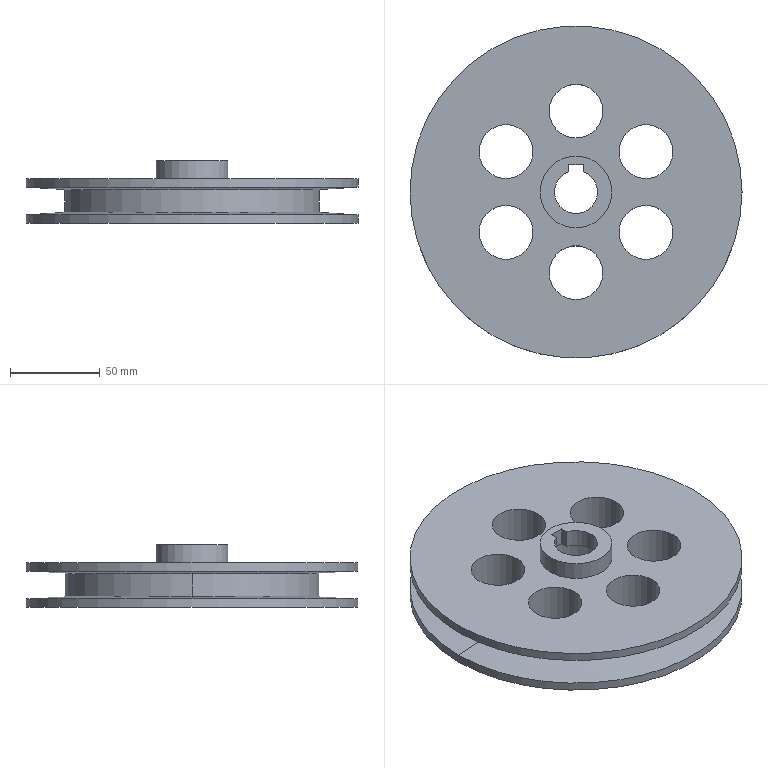Part | NX | features EXTRUDE 2, BREP 1, DATUM_CSYS 1, EXTRACT_DATUM_PLANE 1, INTERSECT 1, SKETCH 1 | 2 solids | 24 faces | box 185 x 185 x 35 mm | volume 385967 mm3 | cylinder 13 | plane 7 | cone 4 | commonest cylinder face diameters 30 x6 40 x2 142 x2 185 x2 24 x1
STEP:
#1=CARTESIAN_POINT('',(20.,0.,-12.5));
#2=VERTEX_POINT('',#1);
#3=CARTESIAN_POINT('',(0.,0.,-12.5));
#4=DIRECTION('',(0.,0.,-1.));
#5=DIRECTION('',(1.,0.,0.));
#6=AXIS2_PLACEMENT_3D('',#3,#4,#5);
#7=CIRCLE('',#6,20.);
#8=EDGE_CURVE('',#2,#2,#7,.T.);
#9=ORIENTED_EDGE('',*,*,#8,.F.);
#10=EDGE_LOOP('',(#9));
#11=FACE_BOUND('',#10,.T.);
#12=CARTESIAN_POINT('',(92.5,0.,-12.5));
#13=VERTEX_POINT('',#12);
#14=CARTESIAN_POINT('',(0.,0.,-12.5));
#15=DIRECTION('',(0.,0.,1.));
#16=DIRECTION('',(1.,0.,0.));
#17=AXIS2_PLACEMENT_3D('',#14,#15,#16);
#18=CIRCLE('',#17,92.5);
#19=EDGE_CURVE('',#13,#13,#18,.T.);
#20=ORIENTED_EDGE('',*,*,#19,.F.);
#21=EDGE_LOOP('',(#20));
#22=FACE_BOUND('',#21,.T.);
#23=CARTESIAN_POINT('',(-15.,45.,-12.5));
#24=VERTEX_POINT('',#23);
#25=CARTESIAN_POINT('',(0.,45.,-12.5));
#26=DIRECTION('',(0.,0.,1.));
#27=DIRECTION('',(-1.,0.,0.));
#28=AXIS2_PLACEMENT_3D('',#25,#26,#27);
#29=CIRCLE('',#28,15.);
#30=EDGE_CURVE('',#24,#24,#29,.T.);
#31=ORIENTED_EDGE('',*,*,#30,.T.);
#32=EDGE_LOOP('',(#31));
#33=FACE_BOUND('',#32,.T.);
#34=CARTESIAN_POINT('',(-53.971,-22.5,-12.5));
#35=VERTEX_POINT('',#34);
#36=CARTESIAN_POINT('',(-38.971,-22.5,-12.5));
#37=DIRECTION('',(0.,0.,1.));
#38=DIRECTION('',(-1.,0.,0.));
#39=AXIS2_PLACEMENT_3D('',#36,#37,#38);
#40=CIRCLE('',#39,15.);
#41=EDGE_CURVE('',#35,#35,#40,.T.);
#42=ORIENTED_EDGE('',*,*,#41,.T.);
#43=EDGE_LOOP('',(#42));
#44=FACE_BOUND('',#43,.T.);
#45=CARTESIAN_POINT('',(23.971,22.5,-12.5));
#46=VERTEX_POINT('',#45);
#47=CARTESIAN_POINT('',(38.971,22.5,-12.5));
#48=DIRECTION('',(0.,0.,1.));
#49=DIRECTION('',(-1.,0.,0.));
#50=AXIS2_PLACEMENT_3D('',#47,#48,#49);
#51=CIRCLE('',#50,15.);
#52=EDGE_CURVE('',#46,#46,#51,.T.);
#53=ORIENTED_EDGE('',*,*,#52,.T.);
#54=EDGE_LOOP('',(#53));
#55=FACE_BOUND('',#54,.T.);
#56=CARTESIAN_POINT('',(23.971,-22.5,-12.5));
#57=VERTEX_POINT('',#56);
#58=CARTESIAN_POINT('',(38.971,-22.5,-12.5));
#59=DIRECTION('',(0.,0.,1.));
#60=DIRECTION('',(-1.,0.,0.));
#61=AXIS2_PLACEMENT_3D('',#58,#59,#60);
#62=CIRCLE('',#61,15.);
#63=EDGE_CURVE('',#57,#57,#62,.T.);
#64=ORIENTED_EDGE('',*,*,#63,.T.);
#65=EDGE_LOOP('',(#64));
#66=FACE_BOUND('',#65,.T.);
#67=CARTESIAN_POINT('',(-15.,-45.,-12.5));
#68=VERTEX_POINT('',#67);
#69=CARTESIAN_POINT('',(0.,-45.,-12.5));
#70=DIRECTION('',(0.,0.,1.));
#71=DIRECTION('',(-1.,0.,0.));
#72=AXIS2_PLACEMENT_3D('',#69,#70,#71);
#73=CIRCLE('',#72,15.);
#74=EDGE_CURVE('',#68,#68,#73,.T.);
#75=ORIENTED_EDGE('',*,*,#74,.T.);
#76=EDGE_LOOP('',(#75));
#77=FACE_BOUND('',#76,.T.);
#78=CARTESIAN_POINT('',(-53.971,22.5,-12.5));
#79=VERTEX_POINT('',#78);
#80=CARTESIAN_POINT('',(-38.971,22.5,-12.5));
#81=DIRECTION('',(0.,0.,1.));
#82=DIRECTION('',(-1.,0.,0.));
#83=AXIS2_PLACEMENT_3D('',#80,#81,#82);
#84=CIRCLE('',#83,15.);
#85=EDGE_CURVE('',#79,#79,#84,.T.);
#86=ORIENTED_EDGE('',*,*,#85,.T.);
#87=EDGE_LOOP('',(#86));
#88=FACE_BOUND('',#87,.T.);
#89=CARTESIAN_POINT('',(0.,0.,-12.5));
#90=DIRECTION('',(0.,0.,1.));
#91=DIRECTION('',(-1.,0.,0.));
#92=AXIS2_PLACEMENT_3D('',#89,#90,#91);
#93=PLANE('',#92);
#94=ADVANCED_FACE('',(#11,#22,#33,#44,#55,#66,#77,#88),#93,.F.);
#95=CARTESIAN_POINT('',(92.5,0.,-7.719));
#96=VERTEX_POINT('',#95);
#97=CARTESIAN_POINT('',(-92.5,0.,-7.719));
#98=VERTEX_POINT('',#97);
#99=CARTESIAN_POINT('',(0.,0.,-7.719));
#100=DIRECTION('',(0.,0.,1.));
#101=DIRECTION('',(1.,0.,0.));
#102=AXIS2_PLACEMENT_3D('',#99,#100,#101);
#103=CIRCLE('',#102,92.5);
#104=EDGE_CURVE('',#96,#98,#103,.T.);
#105=ORIENTED_EDGE('',*,*,#104,.F.);
#106=CARTESIAN_POINT('',(0.,0.,-7.719));
#107=DIRECTION('',(0.,0.,1.));
#108=DIRECTION('',(-1.,0.,0.));
#109=AXIS2_PLACEMENT_3D('',#106,#107,#108);
#110=CIRCLE('',#109,92.5);
#111=EDGE_CURVE('',#98,#96,#110,.T.);
#112=ORIENTED_EDGE('',*,*,#111,.F.);
#113=EDGE_LOOP('',(#105,#112));
#114=FACE_BOUND('',#113,.T.);
#115=ORIENTED_EDGE('',*,*,#19,.T.);
#116=EDGE_LOOP('',(#115));
#117=FACE_BOUND('',#116,.T.);
#118=CARTESIAN_POINT('',(0.,0.,2.5));
#119=DIRECTION('',(0.,0.,1.));
#120=DIRECTION('',(-1.,0.,0.));
#121=AXIS2_PLACEMENT_3D('',#118,#119,#120);
#122=CYLINDRICAL_SURFACE('',#121,92.5);
#123=ADVANCED_FACE('',(#114,#117),#122,.T.);
#124=CARTESIAN_POINT('',(92.5,0.,12.5));
#125=VERTEX_POINT('',#124);
#126=CARTESIAN_POINT('',(0.,0.,12.5));
#127=DIRECTION('',(0.,0.,1.));
#128=DIRECTION('',(1.,0.,0.));
#129=AXIS2_PLACEMENT_3D('',#126,#127,#128);
#130=CIRCLE('',#129,92.5);
#131=EDGE_CURVE('',#125,#125,#130,.T.);
#132=ORIENTED_EDGE('',*,*,#131,.F.);
#133=EDGE_LOOP('',(#132));
#134=FACE_BOUND('',#133,.T.);
#135=CARTESIAN_POINT('',(92.5,0.,7.719));
#136=VERTEX_POINT('',#135);
#137=CARTESIAN_POINT('',(-92.5,0.,7.719));
#138=VERTEX_POINT('',#137);
#139=CARTESIAN_POINT('',(0.,0.,7.719));
#140=DIRECTION('',(0.,0.,1.));
#141=DIRECTION('',(1.,0.,0.));
#142=AXIS2_PLACEMENT_3D('',#139,#140,#141);
#143=CIRCLE('',#142,92.5);
#144=EDGE_CURVE('',#136,#138,#143,.T.);
#145=ORIENTED_EDGE('',*,*,#144,.T.);
#146=CARTESIAN_POINT('',(0.,0.,7.719));
#147=DIRECTION('',(0.,0.,1.));
#148=DIRECTION('',(-1.,0.,0.));
#149=AXIS2_PLACEMENT_3D('',#146,#147,#148);
#150=CIRCLE('',#149,92.5);
#151=EDGE_CURVE('',#138,#136,#150,.T.);
#152=ORIENTED_EDGE('',*,*,#151,.T.);
#153=EDGE_LOOP('',(#145,#152));
#154=FACE_BOUND('',#153,.T.);
#155=CARTESIAN_POINT('',(0.,0.,2.5));
#156=DIRECTION('',(0.,0.,1.));
#157=DIRECTION('',(-1.,0.,0.));
#158=AXIS2_PLACEMENT_3D('',#155,#156,#157);
#159=CYLINDRICAL_SURFACE('',#158,92.5);
#160=ADVANCED_FACE('',(#134,#154),#159,.T.);
#161=CARTESIAN_POINT('',(-71.,0.,-6.381));
#162=VERTEX_POINT('',#161);
#163=CARTESIAN_POINT('',(-92.5,0.,-7.719));
#164=DIRECTION('',(0.9981,0.,0.06213));
#165=VECTOR('',#164,1000.);
#166=LINE('',#163,#165);
#167=EDGE_CURVE('',#98,#162,#166,.T.);
#168=ORIENTED_EDGE('',*,*,#167,.T.);
#169=CARTESIAN_POINT('',(71.,0.,-6.381));
#170=VERTEX_POINT('',#169);
#171=CARTESIAN_POINT('',(0.,0.,-6.381));
#172=DIRECTION('',(0.,0.,1.));
#173=DIRECTION('',(1.,0.,0.));
#174=AXIS2_PLACEMENT_3D('',#171,#172,#173);
#175=CIRCLE('',#174,71.);
#176=EDGE_CURVE('',#170,#162,#175,.T.);
#177=ORIENTED_EDGE('',*,*,#176,.F.);
#178=CARTESIAN_POINT('',(92.5,0.,-7.719));
#179=DIRECTION('',(-0.9981,0.,0.06213));
#180=VECTOR('',#179,1000.);
#181=LINE('',#178,#180);
#182=EDGE_CURVE('',#96,#170,#181,.T.);
#183=ORIENTED_EDGE('',*,*,#182,.F.);
#184=ORIENTED_EDGE('',*,*,#104,.T.);
#185=EDGE_LOOP('',(#168,#177,#183,#184));
#186=FACE_BOUND('',#185,.T.);
#187=CARTESIAN_POINT('',(0.,0.,-7.05));
#188=DIRECTION('',(0.,0.,-1.));
#189=DIRECTION('',(-1.,0.,0.));
#190=AXIS2_PLACEMENT_3D('',#187,#188,#189);
#191=CONICAL_SURFACE('',#190,81.75,1.509);
#192=ADVANCED_FACE('',(#186),#191,.T.);
#193=ORIENTED_EDGE('',*,*,#182,.T.);
#194=CARTESIAN_POINT('',(0.,0.,-6.381));
#195=DIRECTION('',(0.,0.,-1.));
#196=DIRECTION('',(1.,0.,0.));
#197=AXIS2_PLACEMENT_3D('',#194,#195,#196);
#198=CIRCLE('',#197,71.);
#199=EDGE_CURVE('',#170,#162,#198,.T.);
#200=ORIENTED_EDGE('',*,*,#199,.T.);
#201=ORIENTED_EDGE('',*,*,#167,.F.);
#202=ORIENTED_EDGE('',*,*,#111,.T.);
#203=EDGE_LOOP('',(#193,#200,#201,#202));
#204=FACE_BOUND('',#203,.T.);
#205=CARTESIAN_POINT('',(0.,0.,-7.05));
#206=DIRECTION('',(0.,0.,-1.));
#207=DIRECTION('',(-1.,0.,0.));
#208=AXIS2_PLACEMENT_3D('',#205,#206,#207);
#209=CONICAL_SURFACE('',#208,81.75,1.509);
#210=ADVANCED_FACE('',(#204),#209,.T.);
#211=CARTESIAN_POINT('',(-71.,0.,6.381));
#212=VERTEX_POINT('',#211);
#213=CARTESIAN_POINT('',(-71.,0.,6.381));
#214=DIRECTION('',(-0.9981,0.,0.06213));
#215=VECTOR('',#214,1000.);
#216=LINE('',#213,#215);
#217=EDGE_CURVE('',#138,#212,#216,.F.);
#218=ORIENTED_EDGE('',*,*,#217,.T.);
#219=CARTESIAN_POINT('',(71.,0.,6.381));
#220=VERTEX_POINT('',#219);
#221=CARTESIAN_POINT('',(0.,0.,6.381));
#222=DIRECTION('',(0.,0.,-1.));
#223=DIRECTION('',(1.,0.,0.));
#224=AXIS2_PLACEMENT_3D('',#221,#222,#223);
#225=CIRCLE('',#224,71.);
#226=EDGE_CURVE('',#220,#212,#225,.T.);
#227=ORIENTED_EDGE('',*,*,#226,.F.);
#228=CARTESIAN_POINT('',(71.,0.,6.381));
#229=DIRECTION('',(0.9981,0.,0.06213));
#230=VECTOR('',#229,1000.);
#231=LINE('',#228,#230);
#232=EDGE_CURVE('',#136,#220,#231,.F.);
#233=ORIENTED_EDGE('',*,*,#232,.F.);
#234=ORIENTED_EDGE('',*,*,#151,.F.);
#235=EDGE_LOOP('',(#218,#227,#233,#234));
#236=FACE_BOUND('',#235,.T.);
#237=CARTESIAN_POINT('',(0.,0.,7.05));
#238=DIRECTION('',(0.,0.,1.));
#239=DIRECTION('',(1.,0.,0.));
#240=AXIS2_PLACEMENT_3D('',#237,#238,#239);
#241=CONICAL_SURFACE('',#240,81.75,1.509);
#242=ADVANCED_FACE('',(#236),#241,.T.);
#243=ORIENTED_EDGE('',*,*,#232,.T.);
#244=CARTESIAN_POINT('',(0.,0.,6.381));
#245=DIRECTION('',(0.,0.,1.));
#246=DIRECTION('',(1.,0.,0.));
#247=AXIS2_PLACEMENT_3D('',#244,#245,#246);
#248=CIRCLE('',#247,71.);
#249=EDGE_CURVE('',#220,#212,#248,.T.);
#250=ORIENTED_EDGE('',*,*,#249,.T.);
#251=ORIENTED_EDGE('',*,*,#217,.F.);
#252=ORIENTED_EDGE('',*,*,#144,.F.);
#253=EDGE_LOOP('',(#243,#250,#251,#252));
#254=FACE_BOUND('',#253,.T.);
#255=CARTESIAN_POINT('',(0.,0.,7.05));
#256=DIRECTION('',(0.,0.,1.));
#257=DIRECTION('',(1.,0.,0.));
#258=AXIS2_PLACEMENT_3D('',#255,#256,#257);
#259=CONICAL_SURFACE('',#258,81.75,1.509);
#260=ADVANCED_FACE('',(#254),#259,.T.);
#261=ORIENTED_EDGE('',*,*,#176,.T.);
#262=CARTESIAN_POINT('',(-71.,0.,-6.381));
#263=DIRECTION('',(0.,0.,1.));
#264=VECTOR('',#263,1000.);
#265=LINE('',#262,#264);
#266=EDGE_CURVE('',#162,#212,#265,.T.);
#267=ORIENTED_EDGE('',*,*,#266,.T.);
#268=ORIENTED_EDGE('',*,*,#249,.F.);
#269=CARTESIAN_POINT('',(71.,0.,-6.381));
#270=DIRECTION('',(0.,0.,1.));
#271=VECTOR('',#270,1000.);
#272=LINE('',#269,#271);
#273=EDGE_CURVE('',#170,#220,#272,.T.);
#274=ORIENTED_EDGE('',*,*,#273,.F.);
#275=EDGE_LOOP('',(#261,#267,#268,#274));
#276=FACE_BOUND('',#275,.T.);
#277=CARTESIAN_POINT('',(0.,0.,9.35));
#278=DIRECTION('',(0.,0.,-1.));
#279=DIRECTION('',(-1.,0.,0.));
#280=AXIS2_PLACEMENT_3D('',#277,#278,#279);
#281=CYLINDRICAL_SURFACE('',#280,71.);
#282=ADVANCED_FACE('',(#276),#281,.T.);
#283=ORIENTED_EDGE('',*,*,#226,.T.);
#284=ORIENTED_EDGE('',*,*,#266,.F.);
#285=ORIENTED_EDGE('',*,*,#199,.F.);
#286=ORIENTED_EDGE('',*,*,#273,.T.);
#287=EDGE_LOOP('',(#283,#284,#285,#286));
#288=FACE_BOUND('',#287,.T.);
#289=CARTESIAN_POINT('',(0.,0.,9.35));
#290=DIRECTION('',(0.,0.,-1.));
#291=DIRECTION('',(-1.,0.,0.));
#292=AXIS2_PLACEMENT_3D('',#289,#290,#291);
#293=CYLINDRICAL_SURFACE('',#292,71.);
#294=ADVANCED_FACE('',(#288),#293,.T.);
#295=ORIENTED_EDGE('',*,*,#131,.T.);
#296=EDGE_LOOP('',(#295));
#297=FACE_BOUND('',#296,.T.);
#298=CARTESIAN_POINT('',(20.,0.,12.5));
#299=VERTEX_POINT('',#298);
#300=CARTESIAN_POINT('',(0.,0.,12.5));
#301=DIRECTION('',(0.,0.,-1.));
#302=DIRECTION('',(1.,0.,0.));
#303=AXIS2_PLACEMENT_3D('',#300,#301,#302);
#304=CIRCLE('',#303,20.);
#305=EDGE_CURVE('',#299,#299,#304,.T.);
#306=ORIENTED_EDGE('',*,*,#305,.T.);
#307=EDGE_LOOP('',(#306));
#308=FACE_BOUND('',#307,.T.);
#309=CARTESIAN_POINT('',(15.,-45.,12.5));
#310=VERTEX_POINT('',#309);
#311=CARTESIAN_POINT('',(0.,-45.,12.5));
#312=DIRECTION('',(0.,0.,-1.));
#313=DIRECTION('',(1.,0.,0.));
#314=AXIS2_PLACEMENT_3D('',#311,#312,#313);
#315=CIRCLE('',#314,15.);
#316=EDGE_CURVE('',#310,#310,#315,.T.);
#317=ORIENTED_EDGE('',*,*,#316,.T.);
#318=EDGE_LOOP('',(#317));
#319=FACE_BOUND('',#318,.T.);
#320=CARTESIAN_POINT('',(53.971,22.5,12.5));
#321=VERTEX_POINT('',#320);
#322=CARTESIAN_POINT('',(38.971,22.5,12.5));
#323=DIRECTION('',(0.,0.,-1.));
#324=DIRECTION('',(1.,0.,0.));
#325=AXIS2_PLACEMENT_3D('',#322,#323,#324);
#326=CIRCLE('',#325,15.);
#327=EDGE_CURVE('',#321,#321,#326,.T.);
#328=ORIENTED_EDGE('',*,*,#327,.T.);
#329=EDGE_LOOP('',(#328));
#330=FACE_BOUND('',#329,.T.);
#331=CARTESIAN_POINT('',(15.,45.,12.5));
#332=VERTEX_POINT('',#331);
#333=CARTESIAN_POINT('',(0.,45.,12.5));
#334=DIRECTION('',(0.,0.,-1.));
#335=DIRECTION('',(1.,0.,0.));
#336=AXIS2_PLACEMENT_3D('',#333,#334,#335);
#337=CIRCLE('',#336,15.);
#338=EDGE_CURVE('',#332,#332,#337,.T.);
#339=ORIENTED_EDGE('',*,*,#338,.T.);
#340=EDGE_LOOP('',(#339));
#341=FACE_BOUND('',#340,.T.);
#342=CARTESIAN_POINT('',(-23.971,-22.5,12.5));
#343=VERTEX_POINT('',#342);
#344=CARTESIAN_POINT('',(-38.971,-22.5,12.5));
#345=DIRECTION('',(0.,0.,-1.));
#346=DIRECTION('',(1.,0.,0.));
#347=AXIS2_PLACEMENT_3D('',#344,#345,#346);
#348=CIRCLE('',#347,15.);
#349=EDGE_CURVE('',#343,#343,#348,.T.);
#350=ORIENTED_EDGE('',*,*,#349,.T.);
#351=EDGE_LOOP('',(#350));
#352=FACE_BOUND('',#351,.T.);
#353=CARTESIAN_POINT('',(53.971,-22.5,12.5));
#354=VERTEX_POINT('',#353);
#355=CARTESIAN_POINT('',(38.971,-22.5,12.5));
#356=DIRECTION('',(0.,0.,-1.));
#357=DIRECTION('',(1.,0.,0.));
#358=AXIS2_PLACEMENT_3D('',#355,#356,#357);
#359=CIRCLE('',#358,15.);
#360=EDGE_CURVE('',#354,#354,#359,.T.);
#361=ORIENTED_EDGE('',*,*,#360,.T.);
#362=EDGE_LOOP('',(#361));
#363=FACE_BOUND('',#362,.T.);
#364=CARTESIAN_POINT('',(-23.971,22.5,12.5));
#365=VERTEX_POINT('',#364);
#366=CARTESIAN_POINT('',(-38.971,22.5,12.5));
#367=DIRECTION('',(0.,0.,-1.));
#368=DIRECTION('',(1.,0.,0.));
#369=AXIS2_PLACEMENT_3D('',#366,#367,#368);
#370=CIRCLE('',#369,15.);
#371=EDGE_CURVE('',#365,#365,#370,.T.);
#372=ORIENTED_EDGE('',*,*,#371,.T.);
#373=EDGE_LOOP('',(#372));
#374=FACE_BOUND('',#373,.T.);
#375=CARTESIAN_POINT('',(0.,0.,12.5));
#376=DIRECTION('',(0.,0.,1.));
#377=DIRECTION('',(-1.,0.,0.));
#378=AXIS2_PLACEMENT_3D('',#375,#376,#377);
#379=PLANE('',#378);
#380=ADVANCED_FACE('',(#297,#308,#319,#330,#341,#352,#363,#374),#379,.T.);
#381=ORIENTED_EDGE('',*,*,#316,.F.);
#382=EDGE_LOOP('',(#381));
#383=FACE_BOUND('',#382,.T.);
#384=ORIENTED_EDGE('',*,*,#74,.F.);
#385=EDGE_LOOP('',(#384));
#386=FACE_BOUND('',#385,.T.);
#387=CARTESIAN_POINT('',(0.,-45.,2.5));
#388=DIRECTION('',(0.,0.,-1.));
#389=DIRECTION('',(1.,0.,0.));
#390=AXIS2_PLACEMENT_3D('',#387,#388,#389);
#391=CYLINDRICAL_SURFACE('',#390,15.);
#392=ADVANCED_FACE('',(#383,#386),#391,.F.);
#393=ORIENTED_EDGE('',*,*,#327,.F.);
#394=EDGE_LOOP('',(#393));
#395=FACE_BOUND('',#394,.T.);
#396=ORIENTED_EDGE('',*,*,#52,.F.);
#397=EDGE_LOOP('',(#396));
#398=FACE_BOUND('',#397,.T.);
#399=CARTESIAN_POINT('',(38.971,22.5,2.5));
#400=DIRECTION('',(0.,0.,-1.));
#401=DIRECTION('',(1.,0.,0.));
#402=AXIS2_PLACEMENT_3D('',#399,#400,#401);
#403=CYLINDRICAL_SURFACE('',#402,15.);
#404=ADVANCED_FACE('',(#395,#398),#403,.F.);
#405=ORIENTED_EDGE('',*,*,#338,.F.);
#406=EDGE_LOOP('',(#405));
#407=FACE_BOUND('',#406,.T.);
#408=ORIENTED_EDGE('',*,*,#30,.F.);
#409=EDGE_LOOP('',(#408));
#410=FACE_BOUND('',#409,.T.);
#411=CARTESIAN_POINT('',(0.,45.,2.5));
#412=DIRECTION('',(0.,0.,-1.));
#413=DIRECTION('',(1.,0.,0.));
#414=AXIS2_PLACEMENT_3D('',#411,#412,#413);
#415=CYLINDRICAL_SURFACE('',#414,15.);
#416=ADVANCED_FACE('',(#407,#410),#415,.F.);
#417=ORIENTED_EDGE('',*,*,#349,.F.);
#418=EDGE_LOOP('',(#417));
#419=FACE_BOUND('',#418,.T.);
#420=ORIENTED_EDGE('',*,*,#41,.F.);
#421=EDGE_LOOP('',(#420));
#422=FACE_BOUND('',#421,.T.);
#423=CARTESIAN_POINT('',(-38.971,-22.5,2.5));
#424=DIRECTION('',(0.,0.,-1.));
#425=DIRECTION('',(1.,0.,0.));
#426=AXIS2_PLACEMENT_3D('',#423,#424,#425);
#427=CYLINDRICAL_SURFACE('',#426,15.);
#428=ADVANCED_FACE('',(#419,#422),#427,.F.);
#429=ORIENTED_EDGE('',*,*,#360,.F.);
#430=EDGE_LOOP('',(#429));
#431=FACE_BOUND('',#430,.T.);
#432=ORIENTED_EDGE('',*,*,#63,.F.);
#433=EDGE_LOOP('',(#432));
#434=FACE_BOUND('',#433,.T.);
#435=CARTESIAN_POINT('',(38.971,-22.5,2.5));
#436=DIRECTION('',(0.,0.,-1.));
#437=DIRECTION('',(1.,0.,0.));
#438=AXIS2_PLACEMENT_3D('',#435,#436,#437);
#439=CYLINDRICAL_SURFACE('',#438,15.);
#440=ADVANCED_FACE('',(#431,#434),#439,.F.);
#441=ORIENTED_EDGE('',*,*,#371,.F.);
#442=EDGE_LOOP('',(#441));
#443=FACE_BOUND('',#442,.T.);
#444=ORIENTED_EDGE('',*,*,#85,.F.);
#445=EDGE_LOOP('',(#444));
#446=FACE_BOUND('',#445,.T.);
#447=CARTESIAN_POINT('',(-38.971,22.5,2.5));
#448=DIRECTION('',(0.,0.,-1.));
#449=DIRECTION('',(1.,0.,0.));
#450=AXIS2_PLACEMENT_3D('',#447,#448,#449);
#451=CYLINDRICAL_SURFACE('',#450,15.);
#452=ADVANCED_FACE('',(#443,#446),#451,.F.);
#453=ORIENTED_EDGE('',*,*,#305,.F.);
#454=EDGE_LOOP('',(#453));
#455=FACE_BOUND('',#454,.T.);
#456=ORIENTED_EDGE('',*,*,#8,.T.);
#457=EDGE_LOOP('',(#456));
#458=FACE_BOUND('',#457,.T.);
#459=CARTESIAN_POINT('',(0.,0.,-12.5));
#460=DIRECTION('',(0.,0.,1.));
#461=DIRECTION('',(1.,0.,0.));
#462=AXIS2_PLACEMENT_3D('',#459,#460,#461);
#463=CYLINDRICAL_SURFACE('',#462,20.);
#464=ADVANCED_FACE('',(#455,#458),#463,.F.);
#465=CLOSED_SHELL('',(#94,#123,#160,#192,#210,#242,#260,#282,#294,#380,#392,#404,#416,#428,#440,#452,#464));
#466=MANIFOLD_SOLID_BREP('',#465);
#467=CARTESIAN_POINT('',(-4.,11.314,12.5));
#468=VERTEX_POINT('',#467);
#469=CARTESIAN_POINT('',(-4.,15.3,12.5));
#470=VERTEX_POINT('',#469);
#471=CARTESIAN_POINT('',(-4.,11.314,12.5));
#472=DIRECTION('',(0.,1.,0.));
#473=VECTOR('',#472,1000.);
#474=LINE('',#471,#473);
#475=EDGE_CURVE('',#468,#470,#474,.T.);
#476=ORIENTED_EDGE('',*,*,#475,.T.);
#477=CARTESIAN_POINT('',(-4.,15.3,22.5));
#478=VERTEX_POINT('',#477);
#479=CARTESIAN_POINT('',(-4.,15.3,22.5));
#480=DIRECTION('',(0.,0.,-1.));
#481=VECTOR('',#480,1000.);
#482=LINE('',#479,#481);
#483=EDGE_CURVE('',#478,#470,#482,.T.);
#484=ORIENTED_EDGE('',*,*,#483,.F.);
#485=CARTESIAN_POINT('',(-4.,11.314,22.5));
#486=VERTEX_POINT('',#485);
#487=CARTESIAN_POINT('',(-4.,11.314,22.5));
#488=DIRECTION('',(0.,1.,0.));
#489=VECTOR('',#488,1000.);
#490=LINE('',#487,#489);
#491=EDGE_CURVE('',#486,#478,#490,.T.);
#492=ORIENTED_EDGE('',*,*,#491,.F.);
#493=CARTESIAN_POINT('',(-4.,11.314,22.5));
#494=DIRECTION('',(0.,0.,-1.));
#495=VECTOR('',#494,1000.);
#496=LINE('',#493,#495);
#497=EDGE_CURVE('',#486,#468,#496,.T.);
#498=ORIENTED_EDGE('',*,*,#497,.T.);
#499=EDGE_LOOP('',(#476,#484,#492,#498));
#500=FACE_BOUND('',#499,.T.);
#501=CARTESIAN_POINT('',(-4.,11.314,22.5));
#502=DIRECTION('',(-1.,0.,0.));
#503=DIRECTION('',(0.,0.,1.));
#504=AXIS2_PLACEMENT_3D('',#501,#502,#503);
#505=PLANE('',#504);
#506=ADVANCED_FACE('',(#500),#505,.F.);
#507=CARTESIAN_POINT('',(4.,15.3,12.5));
#508=VERTEX_POINT('',#507);
#509=CARTESIAN_POINT('',(-4.,15.3,12.5));
#510=DIRECTION('',(1.,0.,0.));
#511=VECTOR('',#510,1000.);
#512=LINE('',#509,#511);
#513=EDGE_CURVE('',#470,#508,#512,.T.);
#514=ORIENTED_EDGE('',*,*,#513,.T.);
#515=CARTESIAN_POINT('',(4.,15.3,22.5));
#516=VERTEX_POINT('',#515);
#517=CARTESIAN_POINT('',(4.,15.3,22.5));
#518=DIRECTION('',(0.,0.,-1.));
#519=VECTOR('',#518,1000.);
#520=LINE('',#517,#519);
#521=EDGE_CURVE('',#516,#508,#520,.T.);
#522=ORIENTED_EDGE('',*,*,#521,.F.);
#523=CARTESIAN_POINT('',(-4.,15.3,22.5));
#524=DIRECTION('',(1.,0.,0.));
#525=VECTOR('',#524,1000.);
#526=LINE('',#523,#525);
#527=EDGE_CURVE('',#478,#516,#526,.T.);
#528=ORIENTED_EDGE('',*,*,#527,.F.);
#529=ORIENTED_EDGE('',*,*,#483,.T.);
#530=EDGE_LOOP('',(#514,#522,#528,#529));
#531=FACE_BOUND('',#530,.T.);
#532=CARTESIAN_POINT('',(-4.,15.3,22.5));
#533=DIRECTION('',(0.,1.,0.));
#534=DIRECTION('',(0.,0.,1.));
#535=AXIS2_PLACEMENT_3D('',#532,#533,#534);
#536=PLANE('',#535);
#537=ADVANCED_FACE('',(#531),#536,.F.);
#538=CARTESIAN_POINT('',(4.,11.314,12.5));
#539=VERTEX_POINT('',#538);
#540=CARTESIAN_POINT('',(4.,15.3,12.5));
#541=DIRECTION('',(0.,-1.,0.));
#542=VECTOR('',#541,1000.);
#543=LINE('',#540,#542);
#544=EDGE_CURVE('',#508,#539,#543,.T.);
#545=ORIENTED_EDGE('',*,*,#544,.T.);
#546=CARTESIAN_POINT('',(4.,11.314,22.5));
#547=VERTEX_POINT('',#546);
#548=CARTESIAN_POINT('',(4.,11.314,22.5));
#549=DIRECTION('',(0.,0.,-1.));
#550=VECTOR('',#549,1000.);
#551=LINE('',#548,#550);
#552=EDGE_CURVE('',#547,#539,#551,.T.);
#553=ORIENTED_EDGE('',*,*,#552,.F.);
#554=CARTESIAN_POINT('',(4.,15.3,22.5));
#555=DIRECTION('',(0.,-1.,0.));
#556=VECTOR('',#555,1000.);
#557=LINE('',#554,#556);
#558=EDGE_CURVE('',#516,#547,#557,.T.);
#559=ORIENTED_EDGE('',*,*,#558,.F.);
#560=ORIENTED_EDGE('',*,*,#521,.T.);
#561=EDGE_LOOP('',(#545,#553,#559,#560));
#562=FACE_BOUND('',#561,.T.);
#563=CARTESIAN_POINT('',(4.,15.3,22.5));
#564=DIRECTION('',(1.,0.,0.));
#565=DIRECTION('',(0.,0.,-1.));
#566=AXIS2_PLACEMENT_3D('',#563,#564,#565);
#567=PLANE('',#566);
#568=ADVANCED_FACE('',(#562),#567,.F.);
#569=CARTESIAN_POINT('',(20.,0.,12.5));
#570=VERTEX_POINT('',#569);
#571=CARTESIAN_POINT('',(0.,0.,12.5));
#572=DIRECTION('',(0.,0.,1.));
#573=DIRECTION('',(1.,0.,0.));
#574=AXIS2_PLACEMENT_3D('',#571,#572,#573);
#575=CIRCLE('',#574,20.);
#576=EDGE_CURVE('',#570,#570,#575,.T.);
#577=ORIENTED_EDGE('',*,*,#576,.T.);
#578=EDGE_LOOP('',(#577));
#579=FACE_BOUND('',#578,.T.);
#580=CARTESIAN_POINT('',(-20.,0.,22.5));
#581=VERTEX_POINT('',#580);
#582=CARTESIAN_POINT('',(0.,0.,22.5));
#583=DIRECTION('',(0.,0.,1.));
#584=DIRECTION('',(-1.,0.,0.));
#585=AXIS2_PLACEMENT_3D('',#582,#583,#584);
#586=CIRCLE('',#585,20.);
#587=EDGE_CURVE('',#581,#581,#586,.T.);
#588=ORIENTED_EDGE('',*,*,#587,.F.);
#589=EDGE_LOOP('',(#588));
#590=FACE_BOUND('',#589,.T.);
#591=CARTESIAN_POINT('',(0.,0.,22.5));
#592=DIRECTION('',(0.,0.,-1.));
#593=DIRECTION('',(-1.,0.,0.));
#594=AXIS2_PLACEMENT_3D('',#591,#592,#593);
#595=CYLINDRICAL_SURFACE('',#594,20.);
#596=ADVANCED_FACE('',(#579,#590),#595,.T.);
#597=CARTESIAN_POINT('',(0.,0.,12.5));
#598=DIRECTION('',(0.,0.,-1.));
#599=DIRECTION('',(0.3333,0.9428,0.));
#600=AXIS2_PLACEMENT_3D('',#597,#598,#599);
#601=CIRCLE('',#600,12.);
#602=EDGE_CURVE('',#539,#468,#601,.T.);
#603=ORIENTED_EDGE('',*,*,#602,.T.);
#604=ORIENTED_EDGE('',*,*,#497,.F.);
#605=CARTESIAN_POINT('',(0.,0.,22.5));
#606=DIRECTION('',(0.,0.,-1.));
#607=DIRECTION('',(0.3333,0.9428,0.));
#608=AXIS2_PLACEMENT_3D('',#605,#606,#607);
#609=CIRCLE('',#608,12.);
#610=EDGE_CURVE('',#547,#486,#609,.T.);
#611=ORIENTED_EDGE('',*,*,#610,.F.);
#612=ORIENTED_EDGE('',*,*,#552,.T.);
#613=EDGE_LOOP('',(#603,#604,#611,#612));
#614=FACE_BOUND('',#613,.T.);
#615=CARTESIAN_POINT('',(0.,0.,22.5));
#616=DIRECTION('',(0.,0.,-1.));
#617=DIRECTION('',(-1.,0.,0.));
#618=AXIS2_PLACEMENT_3D('',#615,#616,#617);
#619=CYLINDRICAL_SURFACE('',#618,12.);
#620=ADVANCED_FACE('',(#614),#619,.F.);
#621=ORIENTED_EDGE('',*,*,#587,.T.);
#622=EDGE_LOOP('',(#621));
#623=FACE_BOUND('',#622,.T.);
#624=ORIENTED_EDGE('',*,*,#491,.T.);
#625=ORIENTED_EDGE('',*,*,#527,.T.);
#626=ORIENTED_EDGE('',*,*,#558,.T.);
#627=ORIENTED_EDGE('',*,*,#610,.T.);
#628=EDGE_LOOP('',(#624,#625,#626,#627));
#629=FACE_BOUND('',#628,.T.);
#630=CARTESIAN_POINT('',(0.,0.,22.5));
#631=DIRECTION('',(0.,0.,1.));
#632=DIRECTION('',(1.,0.,0.));
#633=AXIS2_PLACEMENT_3D('',#630,#631,#632);
#634=PLANE('',#633);
#635=ADVANCED_FACE('',(#623,#629),#634,.T.);
#636=ORIENTED_EDGE('',*,*,#576,.F.);
#637=EDGE_LOOP('',(#636));
#638=FACE_BOUND('',#637,.T.);
#639=ORIENTED_EDGE('',*,*,#475,.F.);
#640=ORIENTED_EDGE('',*,*,#602,.F.);
#641=ORIENTED_EDGE('',*,*,#544,.F.);
#642=ORIENTED_EDGE('',*,*,#513,.F.);
#643=EDGE_LOOP('',(#639,#640,#641,#642));
#644=FACE_BOUND('',#643,.T.);
#645=CARTESIAN_POINT('',(0.,0.,12.5));
#646=DIRECTION('',(0.,0.,1.));
#647=DIRECTION('',(1.,0.,0.));
#648=AXIS2_PLACEMENT_3D('',#645,#646,#647);
#649=PLANE('',#648);
#650=ADVANCED_FACE('',(#638,#644),#649,.F.);
#651=CLOSED_SHELL('',(#506,#537,#568,#596,#620,#635,#650));
#652=MANIFOLD_SOLID_BREP('',#651);
#653=(LENGTH_UNIT()NAMED_UNIT(*)SI_UNIT(.MILLI.,.METRE.));
#654=UNCERTAINTY_MEASURE_WITH_UNIT(LENGTH_MEASURE(0.00001),#653,'','');
#655=(NAMED_UNIT(*)PLANE_ANGLE_UNIT()SI_UNIT($,.RADIAN.));
#656=(NAMED_UNIT(*)SI_UNIT($,.STERADIAN.)SOLID_ANGLE_UNIT());
#657=(GEOMETRIC_REPRESENTATION_CONTEXT(3)GLOBAL_UNCERTAINTY_ASSIGNED_CONTEXT((#654))GLOBAL_UNIT_ASSIGNED_CONTEXT((#653,#655,#656))REPRESENTATION_CONTEXT('',''));
#658=ADVANCED_BREP_SHAPE_REPRESENTATION('',(#466,#652),#657);